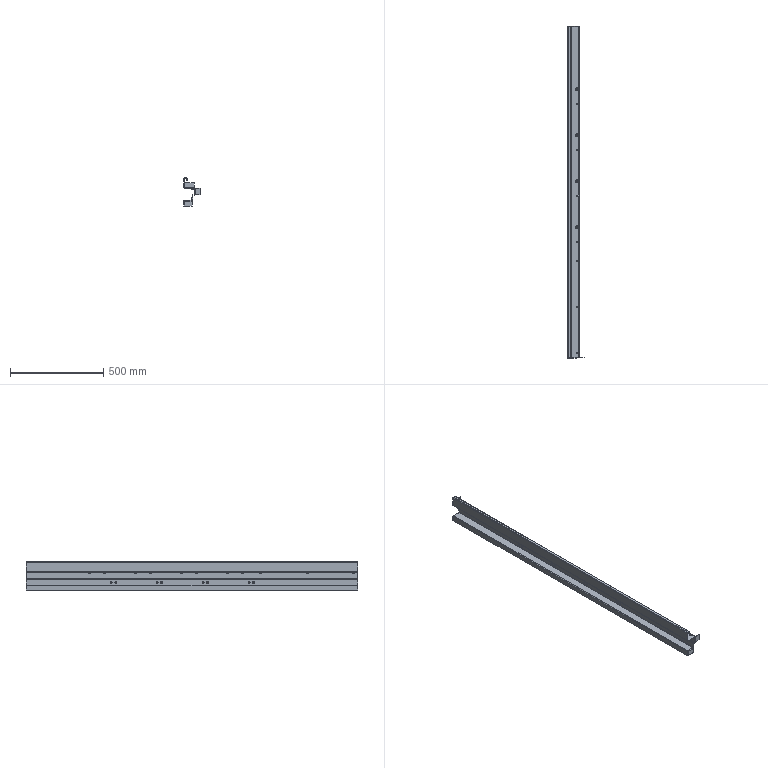Part | SolidWorks | features BaseBody 1 | 1 solid | 368 faces | box 87.5 x 1776 x 150.5 mm | volume 1287455 mm3 | plane 242 | cylinder 126 | commonest cylinder face diameters 6.5 x56 6 x38 2 x12 7 x12 16 x8